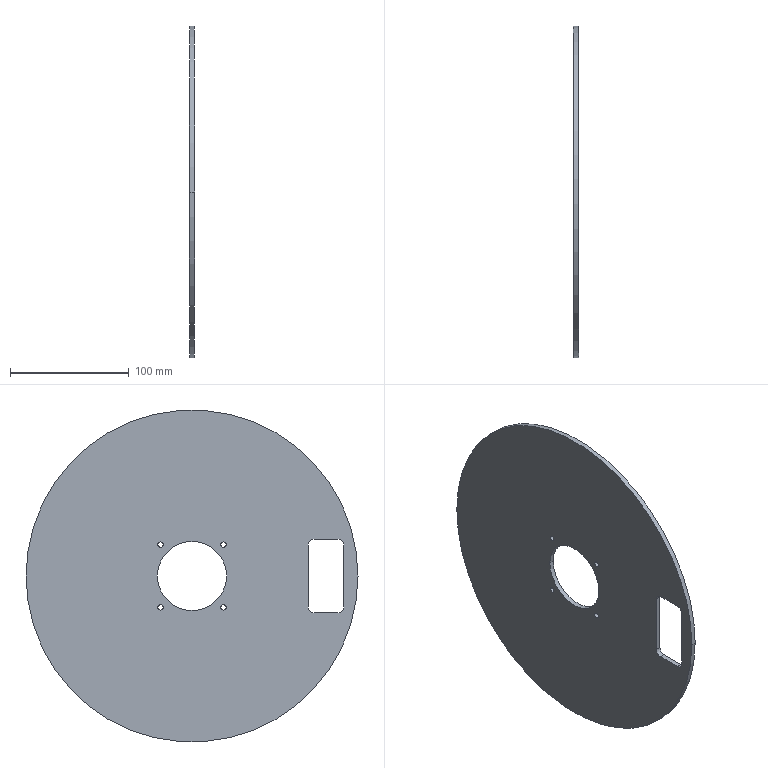Part | SolidWorks | features BaseBody 1 | 1 solid | 22 faces | box 4.269 x 280.004 x 280 mm | volume 227940 mm3 | cylinder 16 | plane 6 | commonest cylinder face diameters 4.5 x8 10 x4 58.5 x2 280 x2
STEP:
#1=CARTESIAN_POINT('',(317.017,325.94,106.919));
#2=VERTEX_POINT('',#1);
#3=CARTESIAN_POINT('',(316.748,605.94,106.919));
#4=VERTEX_POINT('',#3);
#5=CARTESIAN_POINT('',(316.883,465.94,106.919));
#6=DIRECTION('',(1.,0.0009599,0.));
#7=DIRECTION('',(0.0009599,-1.,0.));
#8=AXIS2_PLACEMENT_3D('',#5,#6,#7);
#9=CIRCLE('',#8,140.);
#10=EDGE_CURVE('',#2,#4,#9,.T.);
#11=ORIENTED_EDGE('',*,*,#10,.F.);
#12=CARTESIAN_POINT('',(313.017,325.936,106.919));
#13=VERTEX_POINT('',#12);
#14=CARTESIAN_POINT('',(317.017,325.94,106.919));
#15=DIRECTION('',(-1.,-0.0009599,0.));
#16=VECTOR('',#15,1000.);
#17=LINE('',#14,#16);
#18=EDGE_CURVE('',#2,#13,#17,.T.);
#19=ORIENTED_EDGE('',*,*,#18,.T.);
#20=CARTESIAN_POINT('',(312.748,605.936,106.919));
#21=VERTEX_POINT('',#20);
#22=CARTESIAN_POINT('',(312.883,465.936,106.919));
#23=DIRECTION('',(-1.,-0.0009599,0.));
#24=DIRECTION('',(-0.0009599,1.,0.));
#25=AXIS2_PLACEMENT_3D('',#22,#23,#24);
#26=CIRCLE('',#25,140.);
#27=EDGE_CURVE('',#21,#13,#26,.T.);
#28=ORIENTED_EDGE('',*,*,#27,.F.);
#29=CARTESIAN_POINT('',(316.748,605.94,106.919));
#30=DIRECTION('',(-1.,-0.0009599,0.));
#31=VECTOR('',#30,1000.);
#32=LINE('',#29,#31);
#33=EDGE_CURVE('',#4,#21,#32,.T.);
#34=ORIENTED_EDGE('',*,*,#33,.F.);
#35=EDGE_LOOP('',(#11,#19,#28,#34));
#36=FACE_OUTER_BOUND('',#35,.T.);
#37=CARTESIAN_POINT('',(316.883,465.94,106.919));
#38=DIRECTION('',(-1.,-0.0009599,0.));
#39=DIRECTION('',(-0.0009599,1.,0.));
#40=AXIS2_PLACEMENT_3D('',#37,#38,#39);
#41=CYLINDRICAL_SURFACE('',#40,140.);
#42=ADVANCED_FACE('',(#36),#41,.T.);
#43=CARTESIAN_POINT('',(312.855,494.686,133.419));
#44=VERTEX_POINT('',#43);
#45=CARTESIAN_POINT('',(312.859,490.186,133.419));
#46=VERTEX_POINT('',#45);
#47=CARTESIAN_POINT('',(312.857,492.436,133.419));
#48=DIRECTION('',(1.,0.0009599,0.));
#49=DIRECTION('',(-0.0009599,1.,0.));
#50=AXIS2_PLACEMENT_3D('',#47,#48,#49);
#51=CIRCLE('',#50,2.25);
#52=EDGE_CURVE('',#44,#46,#51,.T.);
#53=ORIENTED_EDGE('',*,*,#52,.F.);
#54=CARTESIAN_POINT('',(316.855,494.69,133.419));
#55=VERTEX_POINT('',#54);
#56=CARTESIAN_POINT('',(316.855,494.69,133.419));
#57=DIRECTION('',(1.,0.0009599,0.));
#58=VECTOR('',#57,1000.);
#59=LINE('',#56,#58);
#60=EDGE_CURVE('',#44,#55,#59,.T.);
#61=ORIENTED_EDGE('',*,*,#60,.T.);
#62=CARTESIAN_POINT('',(316.859,490.19,133.419));
#63=VERTEX_POINT('',#62);
#64=CARTESIAN_POINT('',(316.857,492.44,133.419));
#65=DIRECTION('',(-1.,-0.0009599,0.));
#66=DIRECTION('',(-0.0009599,1.,0.));
#67=AXIS2_PLACEMENT_3D('',#64,#65,#66);
#68=CIRCLE('',#67,2.25);
#69=EDGE_CURVE('',#63,#55,#68,.T.);
#70=ORIENTED_EDGE('',*,*,#69,.F.);
#71=CARTESIAN_POINT('',(316.859,490.19,133.419));
#72=DIRECTION('',(1.,0.0009599,0.));
#73=VECTOR('',#72,1000.);
#74=LINE('',#71,#73);
#75=EDGE_CURVE('',#46,#63,#74,.T.);
#76=ORIENTED_EDGE('',*,*,#75,.F.);
#77=EDGE_LOOP('',(#53,#61,#70,#76));
#78=FACE_OUTER_BOUND('',#77,.T.);
#79=CARTESIAN_POINT('',(316.857,492.44,133.419));
#80=DIRECTION('',(1.,0.0009599,0.));
#81=DIRECTION('',(0.0009599,-1.,0.));
#82=AXIS2_PLACEMENT_3D('',#79,#80,#81);
#83=CYLINDRICAL_SURFACE('',#82,2.25);
#84=ADVANCED_FACE('',(#78),#83,.F.);
#85=CARTESIAN_POINT('',(312.906,441.686,80.419));
#86=VERTEX_POINT('',#85);
#87=CARTESIAN_POINT('',(312.91,437.186,80.419));
#88=VERTEX_POINT('',#87);
#89=CARTESIAN_POINT('',(312.908,439.436,80.419));
#90=DIRECTION('',(1.,0.0009599,0.));
#91=DIRECTION('',(-0.0009599,1.,0.));
#92=AXIS2_PLACEMENT_3D('',#89,#90,#91);
#93=CIRCLE('',#92,2.25);
#94=EDGE_CURVE('',#86,#88,#93,.T.);
#95=ORIENTED_EDGE('',*,*,#94,.F.);
#96=CARTESIAN_POINT('',(316.906,441.69,80.419));
#97=VERTEX_POINT('',#96);
#98=CARTESIAN_POINT('',(316.906,441.69,80.419));
#99=DIRECTION('',(1.,0.0009599,0.));
#100=VECTOR('',#99,1000.);
#101=LINE('',#98,#100);
#102=EDGE_CURVE('',#86,#97,#101,.T.);
#103=ORIENTED_EDGE('',*,*,#102,.T.);
#104=CARTESIAN_POINT('',(316.91,437.19,80.419));
#105=VERTEX_POINT('',#104);
#106=CARTESIAN_POINT('',(316.908,439.44,80.419));
#107=DIRECTION('',(-1.,-0.0009599,0.));
#108=DIRECTION('',(-0.0009599,1.,0.));
#109=AXIS2_PLACEMENT_3D('',#106,#107,#108);
#110=CIRCLE('',#109,2.25);
#111=EDGE_CURVE('',#105,#97,#110,.T.);
#112=ORIENTED_EDGE('',*,*,#111,.F.);
#113=CARTESIAN_POINT('',(316.91,437.19,80.419));
#114=DIRECTION('',(1.,0.0009599,0.));
#115=VECTOR('',#114,1000.);
#116=LINE('',#113,#115);
#117=EDGE_CURVE('',#88,#105,#116,.T.);
#118=ORIENTED_EDGE('',*,*,#117,.F.);
#119=EDGE_LOOP('',(#95,#103,#112,#118));
#120=FACE_OUTER_BOUND('',#119,.T.);
#121=CARTESIAN_POINT('',(316.908,439.44,80.419));
#122=DIRECTION('',(1.,0.0009599,0.));
#123=DIRECTION('',(0.0009599,-1.,0.));
#124=AXIS2_PLACEMENT_3D('',#121,#122,#123);
#125=CYLINDRICAL_SURFACE('',#124,2.25);
#126=ADVANCED_FACE('',(#120),#125,.F.);
#127=CARTESIAN_POINT('',(312.906,441.686,133.419));
#128=VERTEX_POINT('',#127);
#129=CARTESIAN_POINT('',(312.91,437.186,133.419));
#130=VERTEX_POINT('',#129);
#131=CARTESIAN_POINT('',(312.908,439.436,133.419));
#132=DIRECTION('',(1.,0.0009599,0.));
#133=DIRECTION('',(-0.0009599,1.,0.));
#134=AXIS2_PLACEMENT_3D('',#131,#132,#133);
#135=CIRCLE('',#134,2.25);
#136=EDGE_CURVE('',#128,#130,#135,.T.);
#137=ORIENTED_EDGE('',*,*,#136,.F.);
#138=CARTESIAN_POINT('',(316.906,441.69,133.419));
#139=VERTEX_POINT('',#138);
#140=CARTESIAN_POINT('',(316.906,441.69,133.419));
#141=DIRECTION('',(1.,0.0009599,0.));
#142=VECTOR('',#141,1000.);
#143=LINE('',#140,#142);
#144=EDGE_CURVE('',#128,#139,#143,.T.);
#145=ORIENTED_EDGE('',*,*,#144,.T.);
#146=CARTESIAN_POINT('',(316.91,437.19,133.419));
#147=VERTEX_POINT('',#146);
#148=CARTESIAN_POINT('',(316.908,439.44,133.419));
#149=DIRECTION('',(-1.,-0.0009599,0.));
#150=DIRECTION('',(-0.0009599,1.,0.));
#151=AXIS2_PLACEMENT_3D('',#148,#149,#150);
#152=CIRCLE('',#151,2.25);
#153=EDGE_CURVE('',#147,#139,#152,.T.);
#154=ORIENTED_EDGE('',*,*,#153,.F.);
#155=CARTESIAN_POINT('',(316.91,437.19,133.419));
#156=DIRECTION('',(1.,0.0009599,0.));
#157=VECTOR('',#156,1000.);
#158=LINE('',#155,#157);
#159=EDGE_CURVE('',#130,#147,#158,.T.);
#160=ORIENTED_EDGE('',*,*,#159,.F.);
#161=EDGE_LOOP('',(#137,#145,#154,#160));
#162=FACE_OUTER_BOUND('',#161,.T.);
#163=CARTESIAN_POINT('',(316.908,439.44,133.419));
#164=DIRECTION('',(1.,0.0009599,0.));
#165=DIRECTION('',(0.0009599,-1.,0.));
#166=AXIS2_PLACEMENT_3D('',#163,#164,#165);
#167=CYLINDRICAL_SURFACE('',#166,2.25);
#168=ADVANCED_FACE('',(#162),#167,.F.);
#169=CARTESIAN_POINT('',(312.855,494.686,80.419));
#170=VERTEX_POINT('',#169);
#171=CARTESIAN_POINT('',(312.859,490.186,80.419));
#172=VERTEX_POINT('',#171);
#173=CARTESIAN_POINT('',(312.857,492.436,80.419));
#174=DIRECTION('',(1.,0.0009599,0.));
#175=DIRECTION('',(-0.0009599,1.,0.));
#176=AXIS2_PLACEMENT_3D('',#173,#174,#175);
#177=CIRCLE('',#176,2.25);
#178=EDGE_CURVE('',#170,#172,#177,.T.);
#179=ORIENTED_EDGE('',*,*,#178,.F.);
#180=CARTESIAN_POINT('',(316.855,494.69,80.419));
#181=VERTEX_POINT('',#180);
#182=CARTESIAN_POINT('',(316.855,494.69,80.419));
#183=DIRECTION('',(1.,0.0009599,0.));
#184=VECTOR('',#183,1000.);
#185=LINE('',#182,#184);
#186=EDGE_CURVE('',#170,#181,#185,.T.);
#187=ORIENTED_EDGE('',*,*,#186,.T.);
#188=CARTESIAN_POINT('',(316.859,490.19,80.419));
#189=VERTEX_POINT('',#188);
#190=CARTESIAN_POINT('',(316.857,492.44,80.419));
#191=DIRECTION('',(-1.,-0.0009599,0.));
#192=DIRECTION('',(-0.0009599,1.,0.));
#193=AXIS2_PLACEMENT_3D('',#190,#191,#192);
#194=CIRCLE('',#193,2.25);
#195=EDGE_CURVE('',#189,#181,#194,.T.);
#196=ORIENTED_EDGE('',*,*,#195,.F.);
#197=CARTESIAN_POINT('',(316.859,490.19,80.419));
#198=DIRECTION('',(1.,0.0009599,0.));
#199=VECTOR('',#198,1000.);
#200=LINE('',#197,#199);
#201=EDGE_CURVE('',#172,#189,#200,.T.);
#202=ORIENTED_EDGE('',*,*,#201,.F.);
#203=EDGE_LOOP('',(#179,#187,#196,#202));
#204=FACE_OUTER_BOUND('',#203,.T.);
#205=CARTESIAN_POINT('',(316.857,492.44,80.419));
#206=DIRECTION('',(1.,0.0009599,0.));
#207=DIRECTION('',(0.0009599,-1.,0.));
#208=AXIS2_PLACEMENT_3D('',#205,#206,#207);
#209=CYLINDRICAL_SURFACE('',#208,2.25);
#210=ADVANCED_FACE('',(#204),#209,.F.);
#211=CARTESIAN_POINT('',(312.855,495.186,106.919));
#212=VERTEX_POINT('',#211);
#213=CARTESIAN_POINT('',(312.911,436.686,106.919));
#214=VERTEX_POINT('',#213);
#215=CARTESIAN_POINT('',(312.883,465.936,106.919));
#216=DIRECTION('',(1.,0.0009599,0.));
#217=DIRECTION('',(-0.0009599,1.,0.));
#218=AXIS2_PLACEMENT_3D('',#215,#216,#217);
#219=CIRCLE('',#218,29.25);
#220=EDGE_CURVE('',#212,#214,#219,.T.);
#221=ORIENTED_EDGE('',*,*,#220,.F.);
#222=CARTESIAN_POINT('',(316.855,495.19,106.919));
#223=VERTEX_POINT('',#222);
#224=CARTESIAN_POINT('',(312.855,495.186,106.919));
#225=DIRECTION('',(1.,0.0009599,0.));
#226=VECTOR('',#225,1000.);
#227=LINE('',#224,#226);
#228=EDGE_CURVE('',#212,#223,#227,.T.);
#229=ORIENTED_EDGE('',*,*,#228,.T.);
#230=CARTESIAN_POINT('',(316.911,436.69,106.919));
#231=VERTEX_POINT('',#230);
#232=CARTESIAN_POINT('',(316.883,465.94,106.919));
#233=DIRECTION('',(-1.,-0.0009599,0.));
#234=DIRECTION('',(-0.0009599,1.,0.));
#235=AXIS2_PLACEMENT_3D('',#232,#233,#234);
#236=CIRCLE('',#235,29.25);
#237=EDGE_CURVE('',#231,#223,#236,.T.);
#238=ORIENTED_EDGE('',*,*,#237,.F.);
#239=CARTESIAN_POINT('',(312.911,436.686,106.919));
#240=DIRECTION('',(1.,0.0009599,0.));
#241=VECTOR('',#240,1000.);
#242=LINE('',#239,#241);
#243=EDGE_CURVE('',#214,#231,#242,.T.);
#244=ORIENTED_EDGE('',*,*,#243,.F.);
#245=EDGE_LOOP('',(#221,#229,#238,#244));
#246=FACE_OUTER_BOUND('',#245,.T.);
#247=CARTESIAN_POINT('',(312.883,465.936,106.919));
#248=DIRECTION('',(1.,0.0009599,0.));
#249=DIRECTION('',(0.0009599,-1.,0.));
#250=AXIS2_PLACEMENT_3D('',#247,#248,#249);
#251=CYLINDRICAL_SURFACE('',#250,29.25);
#252=ADVANCED_FACE('',(#246),#251,.F.);
#253=ORIENTED_EDGE('',*,*,#228,.F.);
#254=CARTESIAN_POINT('',(312.883,465.936,106.919));
#255=DIRECTION('',(1.,0.0009599,0.));
#256=DIRECTION('',(-0.0009599,1.,0.));
#257=AXIS2_PLACEMENT_3D('',#254,#255,#256);
#258=CIRCLE('',#257,29.25);
#259=EDGE_CURVE('',#214,#212,#258,.T.);
#260=ORIENTED_EDGE('',*,*,#259,.F.);
#261=ORIENTED_EDGE('',*,*,#243,.T.);
#262=CARTESIAN_POINT('',(316.883,465.94,106.919));
#263=DIRECTION('',(-1.,-0.0009599,0.));
#264=DIRECTION('',(-0.0009599,1.,0.));
#265=AXIS2_PLACEMENT_3D('',#262,#263,#264);
#266=CIRCLE('',#265,29.25);
#267=EDGE_CURVE('',#223,#231,#266,.T.);
#268=ORIENTED_EDGE('',*,*,#267,.F.);
#269=EDGE_LOOP('',(#253,#260,#261,#268));
#270=FACE_OUTER_BOUND('',#269,.T.);
#271=CARTESIAN_POINT('',(312.883,465.936,106.919));
#272=DIRECTION('',(1.,0.0009599,0.));
#273=DIRECTION('',(0.0009599,-1.,0.));
#274=AXIS2_PLACEMENT_3D('',#271,#272,#273);
#275=CYLINDRICAL_SURFACE('',#274,29.25);
#276=ADVANCED_FACE('',(#270),#275,.F.);
#277=ORIENTED_EDGE('',*,*,#186,.F.);
#278=CARTESIAN_POINT('',(312.857,492.436,80.419));
#279=DIRECTION('',(1.,0.0009599,0.));
#280=DIRECTION('',(-0.0009599,1.,0.));
#281=AXIS2_PLACEMENT_3D('',#278,#279,#280);
#282=CIRCLE('',#281,2.25);
#283=EDGE_CURVE('',#172,#170,#282,.T.);
#284=ORIENTED_EDGE('',*,*,#283,.F.);
#285=ORIENTED_EDGE('',*,*,#201,.T.);
#286=CARTESIAN_POINT('',(316.857,492.44,80.419));
#287=DIRECTION('',(-1.,-0.0009599,0.));
#288=DIRECTION('',(-0.0009599,1.,0.));
#289=AXIS2_PLACEMENT_3D('',#286,#287,#288);
#290=CIRCLE('',#289,2.25);
#291=EDGE_CURVE('',#181,#189,#290,.T.);
#292=ORIENTED_EDGE('',*,*,#291,.F.);
#293=EDGE_LOOP('',(#277,#284,#285,#292));
#294=FACE_OUTER_BOUND('',#293,.T.);
#295=CARTESIAN_POINT('',(316.857,492.44,80.419));
#296=DIRECTION('',(1.,0.0009599,0.));
#297=DIRECTION('',(0.0009599,-1.,0.));
#298=AXIS2_PLACEMENT_3D('',#295,#296,#297);
#299=CYLINDRICAL_SURFACE('',#298,2.25);
#300=ADVANCED_FACE('',(#294),#299,.F.);
#301=ORIENTED_EDGE('',*,*,#144,.F.);
#302=CARTESIAN_POINT('',(312.908,439.436,133.419));
#303=DIRECTION('',(1.,0.0009599,0.));
#304=DIRECTION('',(-0.0009599,1.,0.));
#305=AXIS2_PLACEMENT_3D('',#302,#303,#304);
#306=CIRCLE('',#305,2.25);
#307=EDGE_CURVE('',#130,#128,#306,.T.);
#308=ORIENTED_EDGE('',*,*,#307,.F.);
#309=ORIENTED_EDGE('',*,*,#159,.T.);
#310=CARTESIAN_POINT('',(316.908,439.44,133.419));
#311=DIRECTION('',(-1.,-0.0009599,0.));
#312=DIRECTION('',(-0.0009599,1.,0.));
#313=AXIS2_PLACEMENT_3D('',#310,#311,#312);
#314=CIRCLE('',#313,2.25);
#315=EDGE_CURVE('',#139,#147,#314,.T.);
#316=ORIENTED_EDGE('',*,*,#315,.F.);
#317=EDGE_LOOP('',(#301,#308,#309,#316));
#318=FACE_OUTER_BOUND('',#317,.T.);
#319=CARTESIAN_POINT('',(316.908,439.44,133.419));
#320=DIRECTION('',(1.,0.0009599,0.));
#321=DIRECTION('',(0.0009599,-1.,0.));
#322=AXIS2_PLACEMENT_3D('',#319,#320,#321);
#323=CYLINDRICAL_SURFACE('',#322,2.25);
#324=ADVANCED_FACE('',(#318),#323,.F.);
#325=ORIENTED_EDGE('',*,*,#102,.F.);
#326=CARTESIAN_POINT('',(312.908,439.436,80.419));
#327=DIRECTION('',(1.,0.0009599,0.));
#328=DIRECTION('',(-0.0009599,1.,0.));
#329=AXIS2_PLACEMENT_3D('',#326,#327,#328);
#330=CIRCLE('',#329,2.25);
#331=EDGE_CURVE('',#88,#86,#330,.T.);
#332=ORIENTED_EDGE('',*,*,#331,.F.);
#333=ORIENTED_EDGE('',*,*,#117,.T.);
#334=CARTESIAN_POINT('',(316.908,439.44,80.419));
#335=DIRECTION('',(-1.,-0.0009599,0.));
#336=DIRECTION('',(-0.0009599,1.,0.));
#337=AXIS2_PLACEMENT_3D('',#334,#335,#336);
#338=CIRCLE('',#337,2.25);
#339=EDGE_CURVE('',#97,#105,#338,.T.);
#340=ORIENTED_EDGE('',*,*,#339,.F.);
#341=EDGE_LOOP('',(#325,#332,#333,#340));
#342=FACE_OUTER_BOUND('',#341,.T.);
#343=CARTESIAN_POINT('',(316.908,439.44,80.419));
#344=DIRECTION('',(1.,0.0009599,0.));
#345=DIRECTION('',(0.0009599,-1.,0.));
#346=AXIS2_PLACEMENT_3D('',#343,#344,#345);
#347=CYLINDRICAL_SURFACE('',#346,2.25);
#348=ADVANCED_FACE('',(#342),#347,.F.);
#349=ORIENTED_EDGE('',*,*,#60,.F.);
#350=CARTESIAN_POINT('',(312.857,492.436,133.419));
#351=DIRECTION('',(1.,0.0009599,0.));
#352=DIRECTION('',(-0.0009599,1.,0.));
#353=AXIS2_PLACEMENT_3D('',#350,#351,#352);
#354=CIRCLE('',#353,2.25);
#355=EDGE_CURVE('',#46,#44,#354,.T.);
#356=ORIENTED_EDGE('',*,*,#355,.F.);
#357=ORIENTED_EDGE('',*,*,#75,.T.);
#358=CARTESIAN_POINT('',(316.857,492.44,133.419));
#359=DIRECTION('',(-1.,-0.0009599,0.));
#360=DIRECTION('',(-0.0009599,1.,0.));
#361=AXIS2_PLACEMENT_3D('',#358,#359,#360);
#362=CIRCLE('',#361,2.25);
#363=EDGE_CURVE('',#55,#63,#362,.T.);
#364=ORIENTED_EDGE('',*,*,#363,.F.);
#365=EDGE_LOOP('',(#349,#356,#357,#364));
#366=FACE_OUTER_BOUND('',#365,.T.);
#367=CARTESIAN_POINT('',(316.857,492.44,133.419));
#368=DIRECTION('',(1.,0.0009599,0.));
#369=DIRECTION('',(0.0009599,-1.,0.));
#370=AXIS2_PLACEMENT_3D('',#367,#368,#369);
#371=CYLINDRICAL_SURFACE('',#370,2.25);
#372=ADVANCED_FACE('',(#366),#371,.F.);
#373=CARTESIAN_POINT('',(317.001,342.94,75.941));
#374=VERTEX_POINT('',#373);
#375=CARTESIAN_POINT('',(313.001,342.936,75.941));
#376=VERTEX_POINT('',#375);
#377=CARTESIAN_POINT('',(317.001,342.94,75.941));
#378=DIRECTION('',(-1.,-0.0009599,0.));
#379=VECTOR('',#378,1000.);
#380=LINE('',#377,#379);
#381=EDGE_CURVE('',#374,#376,#380,.T.);
#382=ORIENTED_EDGE('',*,*,#381,.F.);
#383=CARTESIAN_POINT('',(316.982,362.94,75.941));
#384=VERTEX_POINT('',#383);
#385=CARTESIAN_POINT('',(317.001,342.94,75.941));
#386=DIRECTION('',(-0.0009599,1.,0.));
#387=VECTOR('',#386,1000.);
#388=LINE('',#385,#387);
#389=EDGE_CURVE('',#374,#384,#388,.T.);
#390=ORIENTED_EDGE('',*,*,#389,.T.);
#391=CARTESIAN_POINT('',(312.982,362.936,75.941));
#392=VERTEX_POINT('',#391);
#393=CARTESIAN_POINT('',(312.982,362.936,75.941));
#394=DIRECTION('',(1.,0.0009599,0.));
#395=VECTOR('',#394,1000.);
#396=LINE('',#393,#395);
#397=EDGE_CURVE('',#392,#384,#396,.T.);
#398=ORIENTED_EDGE('',*,*,#397,.F.);
#399=CARTESIAN_POINT('',(313.001,342.936,75.941));
#400=DIRECTION('',(-0.0009599,1.,0.));
#401=VECTOR('',#400,1000.);
#402=LINE('',#399,#401);
#403=EDGE_CURVE('',#376,#392,#402,.T.);
#404=ORIENTED_EDGE('',*,*,#403,.F.);
#405=EDGE_LOOP('',(#382,#390,#398,#404));
#406=FACE_OUTER_BOUND('',#405,.T.);
#407=CARTESIAN_POINT('',(317.001,342.94,75.941));
#408=DIRECTION('',(0.,0.,-1.));
#409=DIRECTION('',(0.,-1.,0.));
#410=AXIS2_PLACEMENT_3D('',#407,#408,#409);
#411=PLANE('',#410);
#412=ADVANCED_FACE('',(#406),#411,.F.);
#413=ORIENTED_EDGE('',*,*,#397,.T.);
#414=CARTESIAN_POINT('',(316.977,367.94,80.941));
#415=VERTEX_POINT('',#414);
#416=CARTESIAN_POINT('',(316.982,362.94,80.941));
#417=DIRECTION('',(-1.,-0.0009599,0.));
#418=DIRECTION('',(-0.0009599,1.,0.));
#419=AXIS2_PLACEMENT_3D('',#416,#417,#418);
#420=CIRCLE('',#419,5.);
#421=EDGE_CURVE('',#415,#384,#420,.T.);
#422=ORIENTED_EDGE('',*,*,#421,.F.);
#423=CARTESIAN_POINT('',(312.977,367.936,80.941));
#424=VERTEX_POINT('',#423);
#425=CARTESIAN_POINT('',(316.977,367.94,80.941));
#426=DIRECTION('',(-1.,-0.0009599,0.));
#427=VECTOR('',#426,1000.);
#428=LINE('',#425,#427);
#429=EDGE_CURVE('',#415,#424,#428,.T.);
#430=ORIENTED_EDGE('',*,*,#429,.T.);
#431=CARTESIAN_POINT('',(312.982,362.936,80.941));
#432=DIRECTION('',(1.,0.0009599,0.));
#433=DIRECTION('',(0.,0.,-1.));
#434=AXIS2_PLACEMENT_3D('',#431,#432,#433);
#435=CIRCLE('',#434,5.);
#436=EDGE_CURVE('',#392,#424,#435,.T.);
#437=ORIENTED_EDGE('',*,*,#436,.F.);
#438=EDGE_LOOP('',(#413,#422,#430,#437));
#439=FACE_OUTER_BOUND('',#438,.T.);
#440=CARTESIAN_POINT('',(316.982,362.94,80.941));
#441=DIRECTION('',(-1.,-0.0009599,0.));
#442=DIRECTION('',(-0.0009599,1.,0.));
#443=AXIS2_PLACEMENT_3D('',#440,#441,#442);
#444=CYLINDRICAL_SURFACE('',#443,5.);
#445=ADVANCED_FACE('',(#439),#444,.F.);
#446=ORIENTED_EDGE('',*,*,#429,.F.);
#447=CARTESIAN_POINT('',(316.977,367.94,132.948));
#448=VERTEX_POINT('',#447);
#449=CARTESIAN_POINT('',(316.977,367.94,80.941));
#450=DIRECTION('',(0.,0.,1.));
#451=VECTOR('',#450,1000.);
#452=LINE('',#449,#451);
#453=EDGE_CURVE('',#415,#448,#452,.T.);
#454=ORIENTED_EDGE('',*,*,#453,.T.);
#455=CARTESIAN_POINT('',(312.977,367.936,132.948));
#456=VERTEX_POINT('',#455);
#457=CARTESIAN_POINT('',(312.977,367.936,132.948));
#458=DIRECTION('',(1.,0.0009599,0.));
#459=VECTOR('',#458,1000.);
#460=LINE('',#457,#459);
#461=EDGE_CURVE('',#456,#448,#460,.T.);
#462=ORIENTED_EDGE('',*,*,#461,.F.);
#463=CARTESIAN_POINT('',(312.977,367.936,80.941));
#464=DIRECTION('',(0.,0.,1.));
#465=VECTOR('',#464,1000.);
#466=LINE('',#463,#465);
#467=EDGE_CURVE('',#424,#456,#466,.T.);
#468=ORIENTED_EDGE('',*,*,#467,.F.);
#469=EDGE_LOOP('',(#446,#454,#462,#468));
#470=FACE_OUTER_BOUND('',#469,.T.);
#471=CARTESIAN_POINT('',(316.977,367.94,132.948));
#472=DIRECTION('',(-0.0009599,1.,0.));
#473=DIRECTION('',(0.,0.,1.));
#474=AXIS2_PLACEMENT_3D('',#471,#472,#473);
#475=PLANE('',#474);
#476=ADVANCED_FACE('',(#470),#475,.F.);
#477=ORIENTED_EDGE('',*,*,#461,.T.);
#478=CARTESIAN_POINT('',(316.982,362.94,137.948));
#479=VERTEX_POINT('',#478);
#480=CARTESIAN_POINT('',(316.982,362.94,132.948));
#481=DIRECTION('',(-1.,-0.0009599,0.));
#482=DIRECTION('',(0.,0.,1.));
#483=AXIS2_PLACEMENT_3D('',#480,#481,#482);
#484=CIRCLE('',#483,5.);
#485=EDGE_CURVE('',#479,#448,#484,.T.);
#486=ORIENTED_EDGE('',*,*,#485,.F.);
#487=CARTESIAN_POINT('',(312.982,362.936,137.948));
#488=VERTEX_POINT('',#487);
#489=CARTESIAN_POINT('',(316.982,362.94,137.948));
#490=DIRECTION('',(-1.,-0.0009599,0.));
#491=VECTOR('',#490,1000.);
#492=LINE('',#489,#491);
#493=EDGE_CURVE('',#479,#488,#492,.T.);
#494=ORIENTED_EDGE('',*,*,#493,.T.);
#495=CARTESIAN_POINT('',(312.982,362.936,132.948));
#496=DIRECTION('',(1.,0.0009599,0.));
#497=DIRECTION('',(-0.0009599,1.,0.));
#498=AXIS2_PLACEMENT_3D('',#495,#496,#497);
#499=CIRCLE('',#498,5.);
#500=EDGE_CURVE('',#456,#488,#499,.T.);
#501=ORIENTED_EDGE('',*,*,#500,.F.);
#502=EDGE_LOOP('',(#477,#486,#494,#501));
#503=FACE_OUTER_BOUND('',#502,.T.);
#504=CARTESIAN_POINT('',(316.982,362.94,132.948));
#505=DIRECTION('',(-1.,-0.0009599,0.));
#506=DIRECTION('',(-0.0009599,1.,0.));
#507=AXIS2_PLACEMENT_3D('',#504,#505,#506);
#508=CYLINDRICAL_SURFACE('',#507,5.);
#509=ADVANCED_FACE('',(#503),#508,.F.);
#510=ORIENTED_EDGE('',*,*,#493,.F.);
#511=CARTESIAN_POINT('',(317.001,342.94,137.948));
#512=VERTEX_POINT('',#511);
#513=CARTESIAN_POINT('',(316.982,362.94,137.948));
#514=DIRECTION('',(0.0009599,-1.,0.));
#515=VECTOR('',#514,1000.);
#516=LINE('',#513,#515);
#517=EDGE_CURVE('',#479,#512,#516,.T.);
#518=ORIENTED_EDGE('',*,*,#517,.T.);
#519=CARTESIAN_POINT('',(313.001,342.936,137.948));
#520=VERTEX_POINT('',#519);
#521=CARTESIAN_POINT('',(313.001,342.936,137.948));
#522=DIRECTION('',(1.,0.0009599,0.));
#523=VECTOR('',#522,1000.);
#524=LINE('',#521,#523);
#525=EDGE_CURVE('',#520,#512,#524,.T.);
#526=ORIENTED_EDGE('',*,*,#525,.F.);
#527=CARTESIAN_POINT('',(312.982,362.936,137.948));
#528=DIRECTION('',(0.0009599,-1.,0.));
#529=VECTOR('',#528,1000.);
#530=LINE('',#527,#529);
#531=EDGE_CURVE('',#488,#520,#530,.T.);
#532=ORIENTED_EDGE('',*,*,#531,.F.);
#533=EDGE_LOOP('',(#510,#518,#526,#532));
#534=FACE_OUTER_BOUND('',#533,.T.);
#535=CARTESIAN_POINT('',(317.001,342.94,137.948));
#536=DIRECTION('',(0.,0.,1.));
#537=DIRECTION('',(1.,0.,0.));
#538=AXIS2_PLACEMENT_3D('',#535,#536,#537);
#539=PLANE('',#538);
#540=ADVANCED_FACE('',(#534),#539,.F.);
#541=ORIENTED_EDGE('',*,*,#525,.T.);
#542=CARTESIAN_POINT('',(317.006,337.94,132.948));
#543=VERTEX_POINT('',#542);
#544=CARTESIAN_POINT('',(317.001,342.94,132.948));
#545=DIRECTION('',(-1.,-0.0009599,0.));
#546=DIRECTION('',(0.0009599,-1.,0.));
#547=AXIS2_PLACEMENT_3D('',#544,#545,#546);
#548=CIRCLE('',#547,5.);
#549=EDGE_CURVE('',#543,#512,#548,.T.);
#550=ORIENTED_EDGE('',*,*,#549,.F.);
#551=CARTESIAN_POINT('',(313.006,337.936,132.948));
#552=VERTEX_POINT('',#551);
#553=CARTESIAN_POINT('',(317.006,337.94,132.948));
#554=DIRECTION('',(-1.,-0.0009599,0.));
#555=VECTOR('',#554,1000.);
#556=LINE('',#553,#555);
#557=EDGE_CURVE('',#543,#552,#556,.T.);
#558=ORIENTED_EDGE('',*,*,#557,.T.);
#559=CARTESIAN_POINT('',(313.001,342.936,132.948));
#560=DIRECTION('',(1.,0.0009599,0.));
#561=DIRECTION('',(0.,0.,1.));
#562=AXIS2_PLACEMENT_3D('',#559,#560,#561);
#563=CIRCLE('',#562,5.);
#564=EDGE_CURVE('',#520,#552,#563,.T.);
#565=ORIENTED_EDGE('',*,*,#564,.F.);
#566=EDGE_LOOP('',(#541,#550,#558,#565));
#567=FACE_OUTER_BOUND('',#566,.T.);
#568=CARTESIAN_POINT('',(317.001,342.94,132.948));
#569=DIRECTION('',(-1.,-0.0009599,0.));
#570=DIRECTION('',(-0.0009599,1.,0.));
#571=AXIS2_PLACEMENT_3D('',#568,#569,#570);
#572=CYLINDRICAL_SURFACE('',#571,5.);
#573=ADVANCED_FACE('',(#567),#572,.F.);
#574=ORIENTED_EDGE('',*,*,#557,.F.);
#575=CARTESIAN_POINT('',(317.006,337.94,80.941));
#576=VERTEX_POINT('',#575);
#577=CARTESIAN_POINT('',(317.006,337.94,132.948));
#578=DIRECTION('',(0.,0.,-1.));
#579=VECTOR('',#578,1000.);
#580=LINE('',#577,#579);
#581=EDGE_CURVE('',#543,#576,#580,.T.);
#582=ORIENTED_EDGE('',*,*,#581,.T.);
#583=CARTESIAN_POINT('',(313.006,337.936,80.941));
#584=VERTEX_POINT('',#583);
#585=CARTESIAN_POINT('',(313.006,337.936,80.941));
#586=DIRECTION('',(1.,0.0009599,0.));
#587=VECTOR('',#586,1000.);
#588=LINE('',#585,#587);
#589=EDGE_CURVE('',#584,#576,#588,.T.);
#590=ORIENTED_EDGE('',*,*,#589,.F.);
#591=CARTESIAN_POINT('',(313.006,337.936,132.948));
#592=DIRECTION('',(0.,0.,-1.));
#593=VECTOR('',#592,1000.);
#594=LINE('',#591,#593);
#595=EDGE_CURVE('',#552,#584,#594,.T.);
#596=ORIENTED_EDGE('',*,*,#595,.F.);
#597=EDGE_LOOP('',(#574,#582,#590,#596));
#598=FACE_OUTER_BOUND('',#597,.T.);
#599=CARTESIAN_POINT('',(317.006,337.94,132.948));
#600=DIRECTION('',(0.0009599,-1.,0.));
#601=DIRECTION('',(0.,0.,-1.));
#602=AXIS2_PLACEMENT_3D('',#599,#600,#601);
#603=PLANE('',#602);
#604=ADVANCED_FACE('',(#598),#603,.F.);
#605=CARTESIAN_POINT('',(313.001,342.936,80.941));
#606=DIRECTION('',(1.,0.0009599,0.));
#607=DIRECTION('',(0.0009599,-1.,0.));
#608=AXIS2_PLACEMENT_3D('',#605,#606,#607);
#609=CIRCLE('',#608,5.);
#610=EDGE_CURVE('',#584,#376,#609,.T.);
#611=ORIENTED_EDGE('',*,*,#610,.T.);
#612=ORIENTED_EDGE('',*,*,#403,.T.);
#613=ORIENTED_EDGE('',*,*,#436,.T.);
#614=ORIENTED_EDGE('',*,*,#467,.T.);
#615=ORIENTED_EDGE('',*,*,#500,.T.);
#616=ORIENTED_EDGE('',*,*,#531,.T.);
#617=ORIENTED_EDGE('',*,*,#564,.T.);
#618=ORIENTED_EDGE('',*,*,#595,.T.);
#619=EDGE_LOOP('',(#611,#612,#613,#614,#615,#616,#617,#618));
#620=FACE_BOUND('',#619,.T.);
#621=ORIENTED_EDGE('',*,*,#259,.T.);
#622=ORIENTED_EDGE('',*,*,#220,.T.);
#623=EDGE_LOOP('',(#621,#622));
#624=FACE_BOUND('',#623,.T.);
#625=ORIENTED_EDGE('',*,*,#283,.T.);
#626=ORIENTED_EDGE('',*,*,#178,.T.);
#627=EDGE_LOOP('',(#625,#626));
#628=FACE_BOUND('',#627,.T.);
#629=ORIENTED_EDGE('',*,*,#307,.T.);
#630=ORIENTED_EDGE('',*,*,#136,.T.);
#631=EDGE_LOOP('',(#629,#630));
#632=FACE_BOUND('',#631,.T.);
#633=ORIENTED_EDGE('',*,*,#331,.T.);
#634=ORIENTED_EDGE('',*,*,#94,.T.);
#635=EDGE_LOOP('',(#633,#634));
#636=FACE_BOUND('',#635,.T.);
#637=ORIENTED_EDGE('',*,*,#355,.T.);
#638=ORIENTED_EDGE('',*,*,#52,.T.);
#639=EDGE_LOOP('',(#637,#638));
#640=FACE_BOUND('',#639,.T.);
#641=ORIENTED_EDGE('',*,*,#27,.T.);
#642=CARTESIAN_POINT('',(312.883,465.936,106.919));
#643=DIRECTION('',(-1.,-0.0009599,0.));
#644=DIRECTION('',(-0.0009599,1.,0.));
#645=AXIS2_PLACEMENT_3D('',#642,#643,#644);
#646=CIRCLE('',#645,140.);
#647=EDGE_CURVE('',#13,#21,#646,.T.);
#648=ORIENTED_EDGE('',*,*,#647,.T.);
#649=EDGE_LOOP('',(#641,#648));
#650=FACE_OUTER_BOUND('',#649,.T.);
#651=CARTESIAN_POINT('',(312.883,465.936,106.919));
#652=DIRECTION('',(1.,0.0009599,0.));
#653=DIRECTION('',(0.,0.,-1.));
#654=AXIS2_PLACEMENT_3D('',#651,#652,#653);
#655=PLANE('',#654);
#656=ADVANCED_FACE('',(#620,#624,#628,#632,#636,#640,#650),#655,.F.);
#657=ORIENTED_EDGE('',*,*,#589,.T.);
#658=CARTESIAN_POINT('',(317.001,342.94,80.941));
#659=DIRECTION('',(-1.,-0.0009599,0.));
#660=DIRECTION('',(0.,0.,-1.));
#661=AXIS2_PLACEMENT_3D('',#658,#659,#660);
#662=CIRCLE('',#661,5.);
#663=EDGE_CURVE('',#374,#576,#662,.T.);
#664=ORIENTED_EDGE('',*,*,#663,.F.);
#665=ORIENTED_EDGE('',*,*,#381,.T.);
#666=ORIENTED_EDGE('',*,*,#610,.F.);
#667=EDGE_LOOP('',(#657,#664,#665,#666));
#668=FACE_OUTER_BOUND('',#667,.T.);
#669=CARTESIAN_POINT('',(317.001,342.94,80.941));
#670=DIRECTION('',(-1.,-0.0009599,0.));
#671=DIRECTION('',(-0.0009599,1.,0.));
#672=AXIS2_PLACEMENT_3D('',#669,#670,#671);
#673=CYLINDRICAL_SURFACE('',#672,5.);
#674=ADVANCED_FACE('',(#668),#673,.F.);
#675=ORIENTED_EDGE('',*,*,#581,.F.);
#676=ORIENTED_EDGE('',*,*,#549,.T.);
#677=ORIENTED_EDGE('',*,*,#517,.F.);
#678=ORIENTED_EDGE('',*,*,#485,.T.);
#679=ORIENTED_EDGE('',*,*,#453,.F.);
#680=ORIENTED_EDGE('',*,*,#421,.T.);
#681=ORIENTED_EDGE('',*,*,#389,.F.);
#682=ORIENTED_EDGE('',*,*,#663,.T.);
#683=EDGE_LOOP('',(#675,#676,#677,#678,#679,#680,#681,#682));
#684=FACE_BOUND('',#683,.T.);
#685=ORIENTED_EDGE('',*,*,#237,.T.);
#686=ORIENTED_EDGE('',*,*,#267,.T.);
#687=EDGE_LOOP('',(#685,#686));
#688=FACE_BOUND('',#687,.T.);
#689=ORIENTED_EDGE('',*,*,#195,.T.);
#690=ORIENTED_EDGE('',*,*,#291,.T.);
#691=EDGE_LOOP('',(#689,#690));
#692=FACE_BOUND('',#691,.T.);
#693=ORIENTED_EDGE('',*,*,#153,.T.);
#694=ORIENTED_EDGE('',*,*,#315,.T.);
#695=EDGE_LOOP('',(#693,#694));
#696=FACE_BOUND('',#695,.T.);
#697=ORIENTED_EDGE('',*,*,#111,.T.);
#698=ORIENTED_EDGE('',*,*,#339,.T.);
#699=EDGE_LOOP('',(#697,#698));
#700=FACE_BOUND('',#699,.T.);
#701=ORIENTED_EDGE('',*,*,#69,.T.);
#702=ORIENTED_EDGE('',*,*,#363,.T.);
#703=EDGE_LOOP('',(#701,#702));
#704=FACE_BOUND('',#703,.T.);
#705=CARTESIAN_POINT('',(316.883,465.94,106.919));
#706=DIRECTION('',(1.,0.0009599,0.));
#707=DIRECTION('',(0.0009599,-1.,0.));
#708=AXIS2_PLACEMENT_3D('',#705,#706,#707);
#709=CIRCLE('',#708,140.);
#710=EDGE_CURVE('',#4,#2,#709,.T.);
#711=ORIENTED_EDGE('',*,*,#710,.T.);
#712=ORIENTED_EDGE('',*,*,#10,.T.);
#713=EDGE_LOOP('',(#711,#712));
#714=FACE_OUTER_BOUND('',#713,.T.);
#715=CARTESIAN_POINT('',(316.883,465.94,106.919));
#716=DIRECTION('',(1.,0.0009599,0.));
#717=DIRECTION('',(0.,0.,-1.));
#718=AXIS2_PLACEMENT_3D('',#715,#716,#717);
#719=PLANE('',#718);
#720=ADVANCED_FACE('',(#684,#688,#692,#696,#700,#704,#714),#719,.T.);
#721=ORIENTED_EDGE('',*,*,#18,.F.);
#722=ORIENTED_EDGE('',*,*,#710,.F.);
#723=ORIENTED_EDGE('',*,*,#33,.T.);
#724=ORIENTED_EDGE('',*,*,#647,.F.);
#725=EDGE_LOOP('',(#721,#722,#723,#724));
#726=FACE_OUTER_BOUND('',#725,.T.);
#727=CARTESIAN_POINT('',(316.883,465.94,106.919));
#728=DIRECTION('',(-1.,-0.0009599,0.));
#729=DIRECTION('',(-0.0009599,1.,0.));
#730=AXIS2_PLACEMENT_3D('',#727,#728,#729);
#731=CYLINDRICAL_SURFACE('',#730,140.);
#732=ADVANCED_FACE('',(#726),#731,.T.);
#733=CLOSED_SHELL('',(#42,#84,#126,#168,#210,#252,#276,#300,#324,#348,#372,#412,#445,#476,#509,#540,#573,#604,#656,#674,#720,#732));
#734=MANIFOLD_SOLID_BREP('',#733);
#735=CARTESIAN_POINT('',(0.,0.,0.));
#736=DIRECTION('',(0.,0.,1.));
#737=DIRECTION('',(1.,0.,0.));
#738=AXIS2_PLACEMENT_3D('',#735,#736,#737);
#739=(LENGTH_UNIT()NAMED_UNIT(*)SI_UNIT(.MILLI.,.METRE.));
#740=UNCERTAINTY_MEASURE_WITH_UNIT(LENGTH_MEASURE(0.00001),#739,'','');
#741=(NAMED_UNIT(*)PLANE_ANGLE_UNIT()SI_UNIT($,.RADIAN.));
#742=(NAMED_UNIT(*)SI_UNIT($,.STERADIAN.)SOLID_ANGLE_UNIT());
#743=(GEOMETRIC_REPRESENTATION_CONTEXT(3)GLOBAL_UNCERTAINTY_ASSIGNED_CONTEXT((#740))GLOBAL_UNIT_ASSIGNED_CONTEXT((#739,#741,#742))REPRESENTATION_CONTEXT('',''));
#744=ADVANCED_BREP_SHAPE_REPRESENTATION('',(#734,#738),#743);